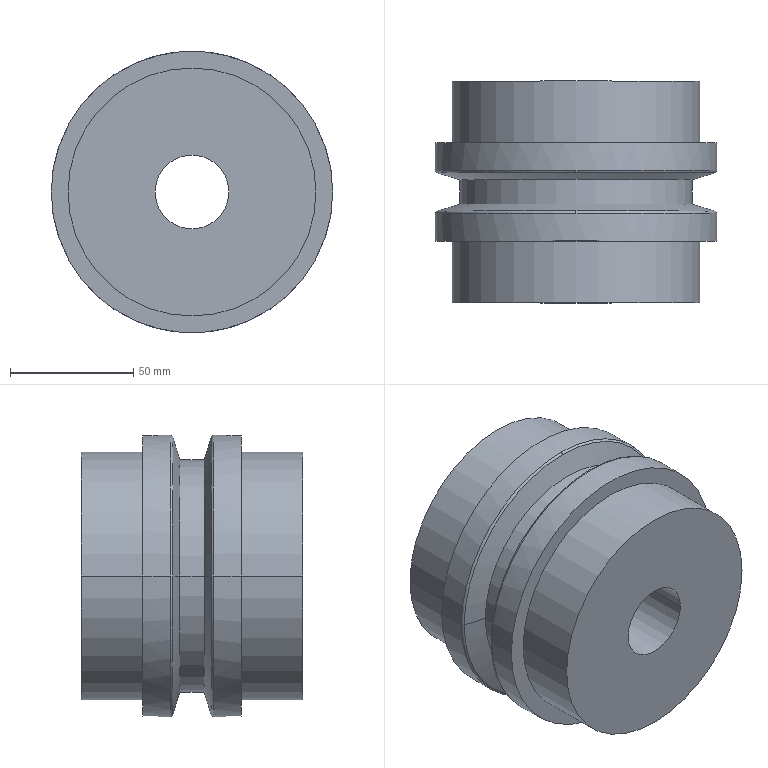Part | STEP file | ROLLER.3.stp | 1 solid | 24 faces | box 114.3 x 90 x 114.3 mm | volume 702058 mm3 | cylinder 12 | plane 4 | torus 4 | cone 4 | commonest cylinder face diameters 100.7 x4 114.3 x4 30 x2 94.3 x2